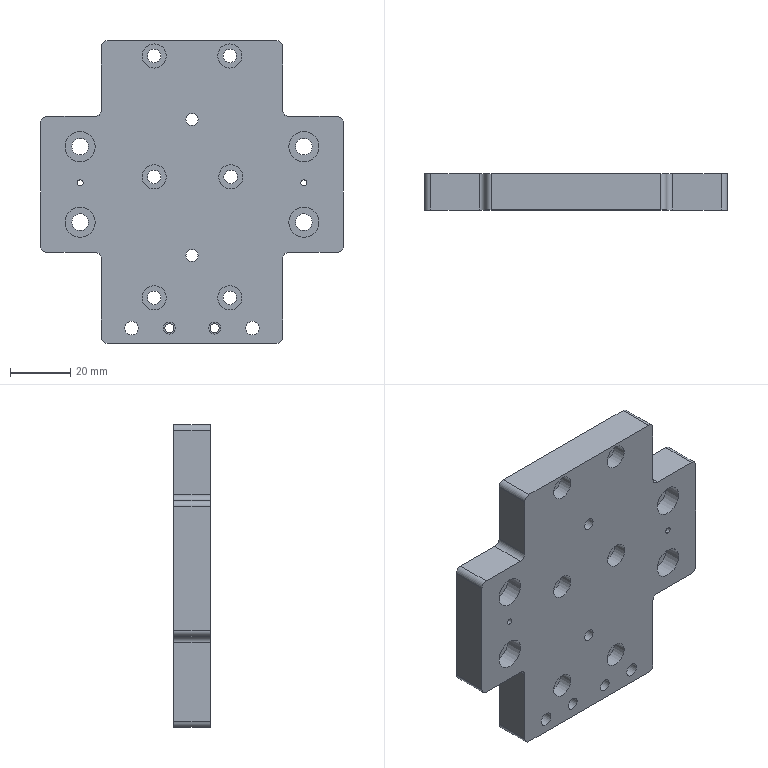Part | STEP file | SynoNew-0304-065 | 1 solid | 78 faces | box 100 x 12 x 100 mm | volume 87539 mm3 | cylinder 47 | plane 30 | cone 1 | commonest cylinder face diameters 4 x18 4.5 x8 8 x8 5.5 x4 10 x4 2 x2